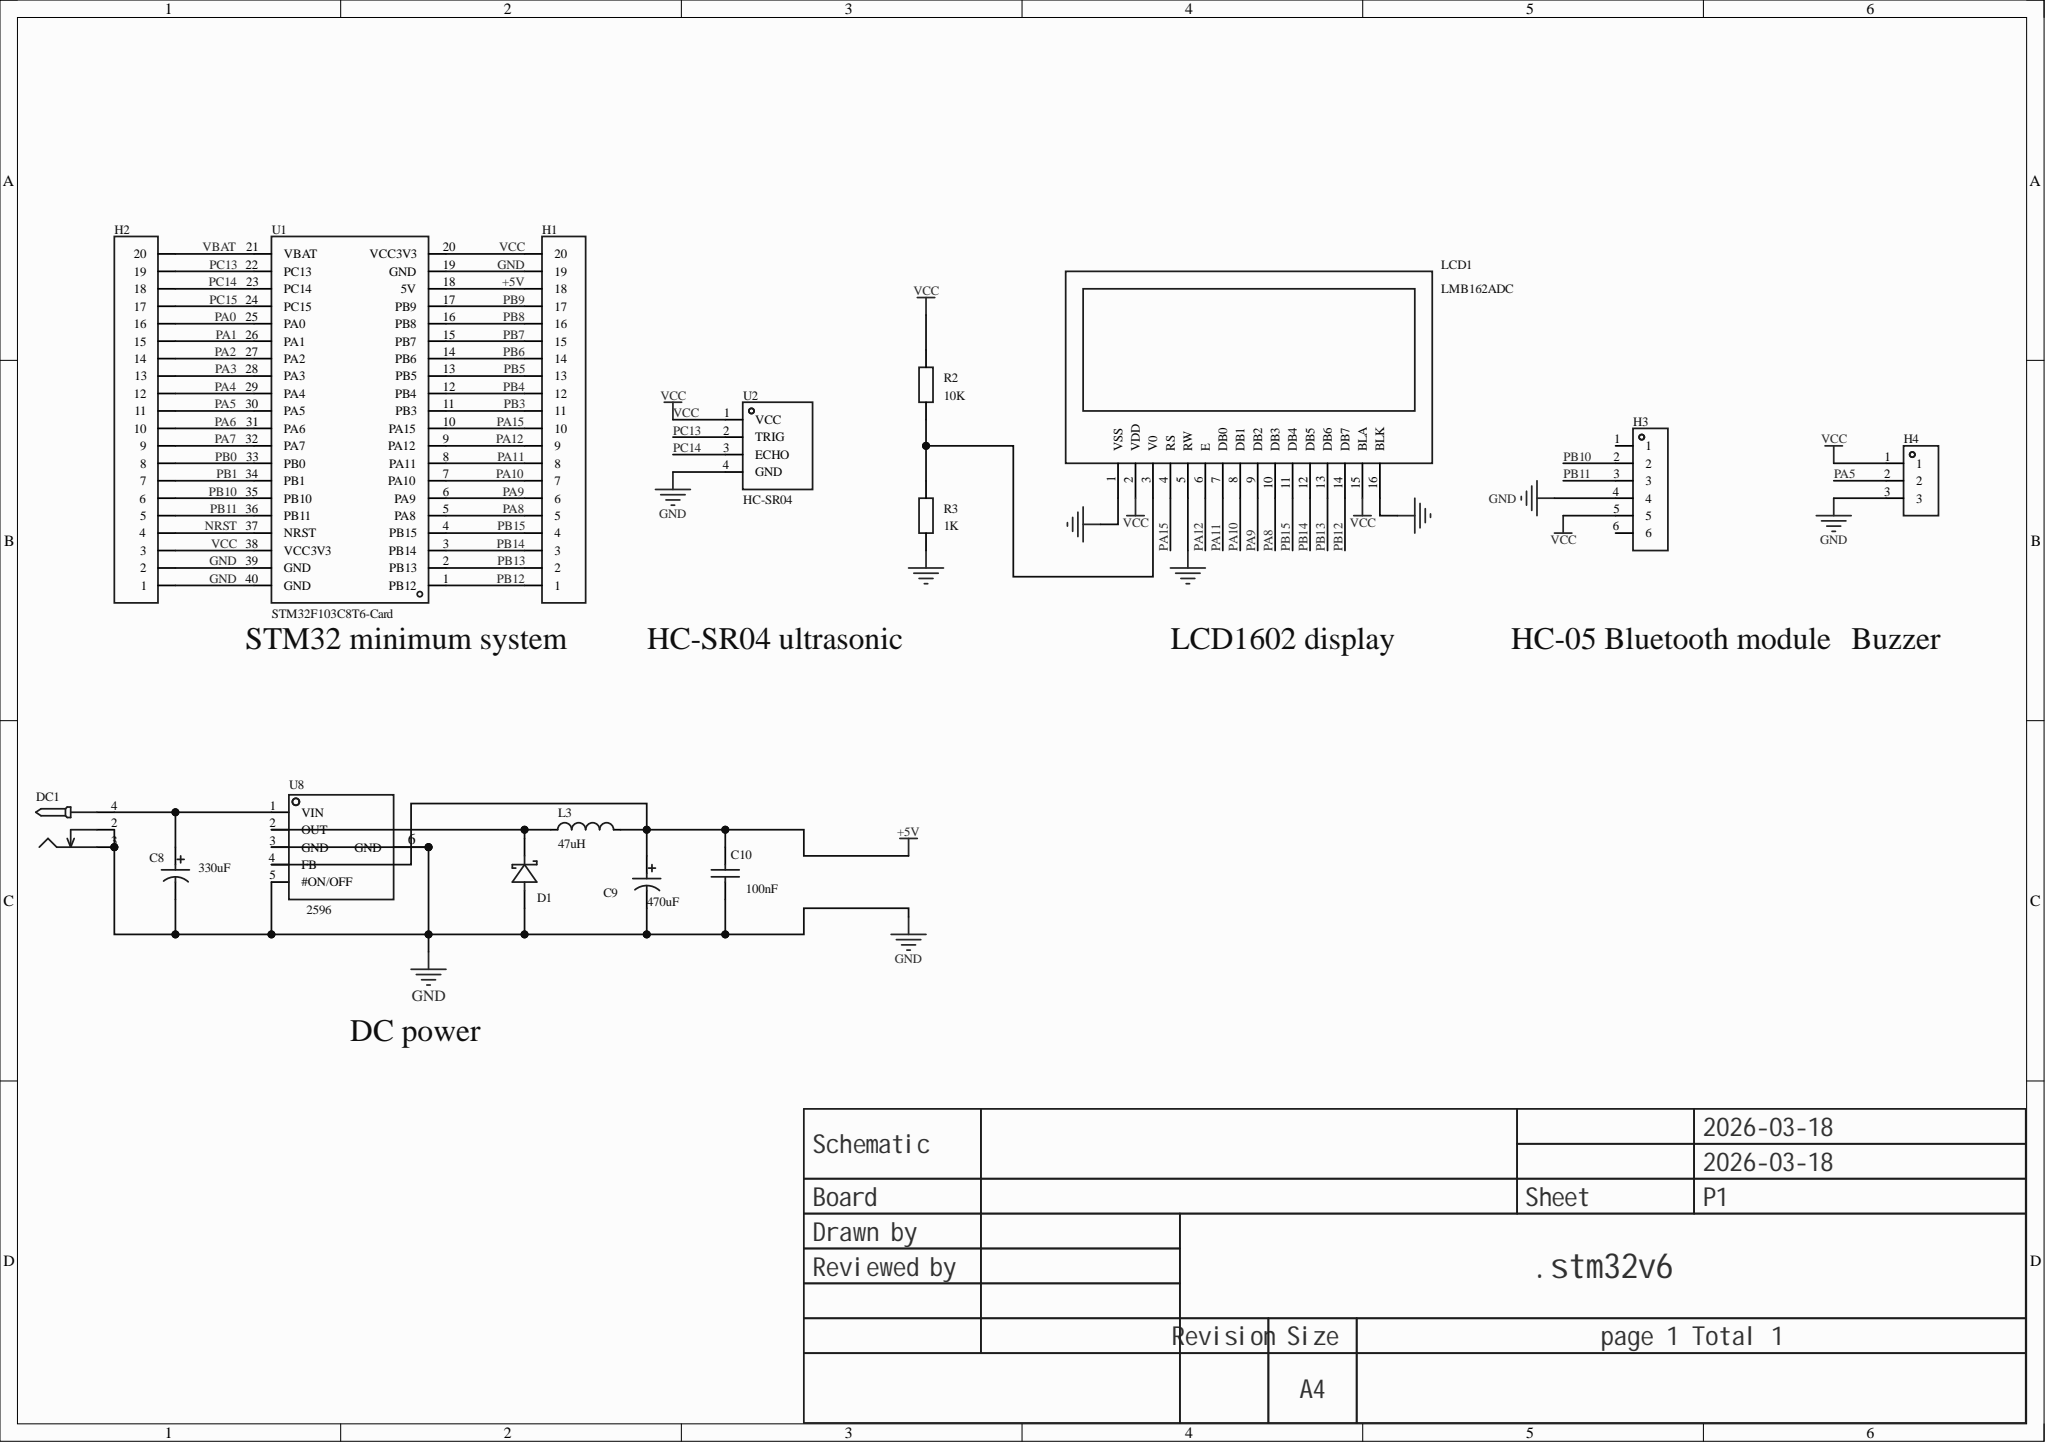Circuit board | Altium Designer | 16 parts | 40 nets
Bill of materials:
Comment,Description,Designator,Footprint,LibRef,Quantity
"","Capacitance: 220uF; tolerance: ±20%; rated voltage: 35V; capacitor body diameter: 8mm; body length: 10.5mm; ripple current: -; ESR: -; operating life: 2000hrs@105; operating temperature: -40~+105;","C8, C9","CAP-SMD_BD8.0-L8.3-W8.3-RD","CS1V221M-CRF10","2"
"","Capacitance: 100nF; tolerance: ±10%; rated voltage: 50V; temperature coefficient: X7R;","C10","C0805","CL21B104KBCNNNC","1"
"","","D1","SMA_L4.3-W2.6-LS5.2-RD","SS34_3","1"
"","","DC1","DC-2.0","DC-005_2.0","1"
"","","H1, H2","HDR-TH_20P-P2.54-V-F","HDR-F_2.54_1x20P","2"
"","","H3","HDR-TH_6P-P2.54-V-F","HDR-F_2.54_1x6P","1"
"","","H4","HDR-TH_3P-P2.54-V-F","HDR-F_2.54_1x3P","1"
"","Inductance: 33uH; tolerance: ±20%; DC resistance (DCR): 270mO;","L3","IND-SMD_L7.0-W6.6","CMLO0630H330MTT","1"
"LMB162ADC","16x2 character LCD module","LCD1","LCD1602","LMB162ADC","1"
"10K","","R2","R0805","Res_0805","1"
"1K","","R3","R0805","Res_0805","1"
"STM32F103C8T6-Card","","U1","CONN-TH_L53.3-W22.9_STM32F103C8T6-CARD","STM32F103C8T6-Card","1"
"HC-SR04","","U2","TH_HC-SR04V","HC-SR04","1"
"LM2596S-5.0","Function type: step-down; output type: fixed; input voltage: 40V; output voltage: 5V; output current (max): 3A;","U8","TO-263-5_L10.2-W8.9-P1.70-BR","LM2596S-5.0_C347421","1"
Netlist (Protel format):
[
C8
CAP-SMD_BD8.0-L8.3-W8.3-RD




]
[
C9
CAP-SMD_BD8.0-L8.3-W8.3-RD




]
[
C10
C0805




]
[
D1
SMA_L4.3-W2.6-LS5.2-RD




]
[
DC1
DC-2.0




]
[
H1
HDR-TH_20P-P2.54-V-F




]
[
H2
HDR-TH_20P-P2.54-V-F




]
[
H3
HDR-TH_6P-P2.54-V-F




]
[
H4
HDR-TH_3P-P2.54-V-F




]
[
L3
IND-SMD_L7.0-W6.6




]
[
LCD1
LCD1602
LMB162ADC



]
[
R2
R0805
10K



]
[
R3
R0805
1K



]
[
U1
CONN-TH_L53.3-W22.9_STM32F103C8T6-CARD
STM32F103C8T6-Card



]
[
U2
TH_HC-SR04V
HC-SR04



]
[
U8
TO-263-5_L10.2-W8.9-P1.70-BR
LM2596S-5.0



]
(
VCC
H1-20
H2-3
H3-5
H4-1
LCD1-2
LCD1-15
R2-2
U1-20
U1-38
U2-1
)
(
VBAT
H2-20
U1-21
)
(
PC15
H2-17
U1-24
)
(
PC14
H2-18
U1-23
U2-3
)
(
PC13
H2-19
U1-22
U2-2
)
(
PB15
H1-4
LCD1-11
U1-4
)
(
PB14
H1-3
LCD1-12
U1-3
)
(
PB13
H1-2
LCD1-13
U1-2
)
(
PB12
H1-1
LCD1-14
U1-1
)
(
PB11
H2-5
H3-3
U1-36
)
(
PB10
H2-6
H3-2
U1-35
)
(
PB9
H1-17
U1-17
)
(
PB8
H1-16
U1-16
)
(
PB7
H1-15
U1-15
)
(
PB6
H1-14
U1-14
)
(
PB5
H1-13
U1-13
)
(
PB4
H1-12
U1-12
)
(
PB3
H1-11
U1-11
)
(
PB1
H2-7
U1-34
)
(
PB0
H2-8
U1-33
)
(
PA15
H1-10
LCD1-4
U1-10
)
(
PA12
H1-9
LCD1-6
U1-9
)
(
PA11
H1-8
LCD1-7
U1-8
)
(
PA10
H1-7
LCD1-8
U1-7
)
(
PA9
H1-6
LCD1-9
U1-6
)
(
PA8
H1-5
LCD1-10
U1-5
)
(
PA7
H2-9
U1-32
)
(
PA6
H2-10
U1-31
)
(
PA5
H2-11
H4-2
U1-30
)
(
PA4
H2-12
U1-29
)
(
PA3
H2-13
U1-28
)
(
PA2
H2-14
U1-27
)
(
PA1
H2-15
U1-26
)
(
PA0
H2-16
U1-25
)
(
NRST
H2-4
U1-37
)
(
NetLCD1_3
LCD1-3
R2-1
R3-2
)
(
NetD1_1
D1-1
L3-1
U8-2
)
(
NetC8_1
C8-1
DC1-4
U8-1
)
(
GND
C8-2
C9-2
C10-2
D1-2
DC1-2
DC1-3
H1-19
H2-1
H2-2
H3-4
H4-3
LCD1-1
LCD1-5
LCD1-16
R3-1
U1-19
U1-39
U1-40
U2-4
U8-3
U8-5
U8-6
)
(
+5V
C9-1
C10-1
H1-18
L3-2
U1-18
U8-4
)